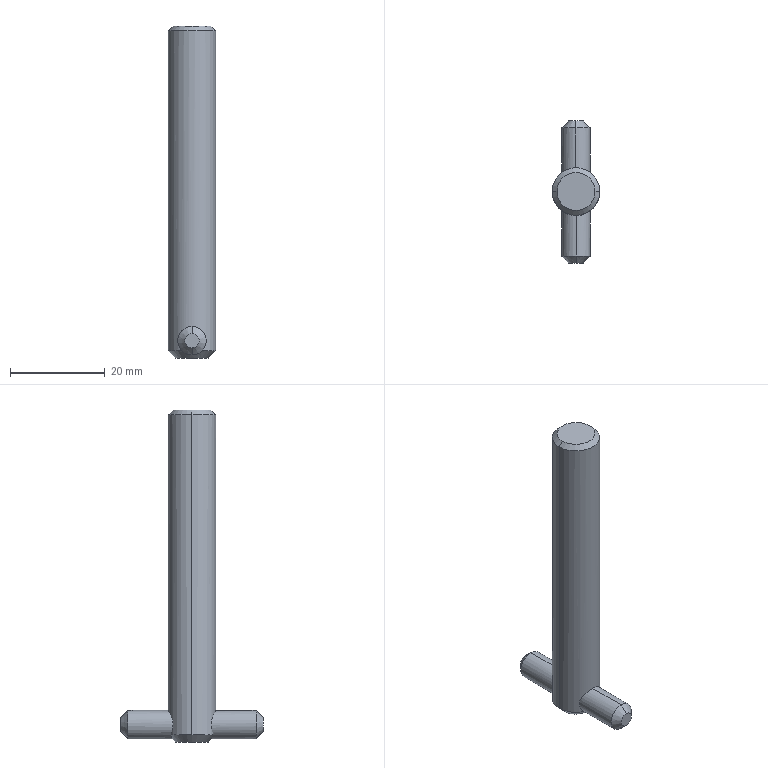Part | SolidWorks | features Chamfer 2, Extrusion 1, ICE 1 | 1 solid | 18 faces | box 10 x 30 x 70 mm | volume 5997 mm3 | cone 8 | cylinder 6 | plane 4 | commonest cylinder face diameters 6 x4 10 x2
STEP:
#1=CARTESIAN_POINT('',(4.,0.,70.));
#2=VERTEX_POINT('',#1);
#3=CARTESIAN_POINT('',(-4.,0.,70.));
#4=VERTEX_POINT('',#3);
#5=CARTESIAN_POINT('',(0.,0.,70.));
#6=DIRECTION('',(0.,0.,1.));
#7=DIRECTION('',(1.,0.,0.));
#8=AXIS2_PLACEMENT_3D('',#5,#6,#7);
#9=CIRCLE('',#8,4.);
#10=EDGE_CURVE('',#2,#4,#9,.T.);
#11=ORIENTED_EDGE('',*,*,#10,.F.);
#12=CARTESIAN_POINT('',(5.,0.,69.));
#13=VERTEX_POINT('',#12);
#14=CARTESIAN_POINT('',(4.,0.,70.));
#15=DIRECTION('',(0.7071,0.,-0.7071));
#16=VECTOR('',#15,1000.);
#17=LINE('',#14,#16);
#18=EDGE_CURVE('',#2,#13,#17,.T.);
#19=ORIENTED_EDGE('',*,*,#18,.T.);
#20=CARTESIAN_POINT('',(-5.,0.,69.));
#21=VERTEX_POINT('',#20);
#22=CARTESIAN_POINT('',(0.,0.,69.));
#23=DIRECTION('',(0.,0.,-1.));
#24=DIRECTION('',(1.,0.,0.));
#25=AXIS2_PLACEMENT_3D('',#22,#23,#24);
#26=CIRCLE('',#25,5.);
#27=EDGE_CURVE('',#21,#13,#26,.T.);
#28=ORIENTED_EDGE('',*,*,#27,.F.);
#29=CARTESIAN_POINT('',(-4.,0.,70.));
#30=DIRECTION('',(-0.7071,0.,-0.7071));
#31=VECTOR('',#30,1000.);
#32=LINE('',#29,#31);
#33=EDGE_CURVE('',#4,#21,#32,.T.);
#34=ORIENTED_EDGE('',*,*,#33,.F.);
#35=EDGE_LOOP('',(#11,#19,#28,#34));
#36=FACE_OUTER_BOUND('',#35,.T.);
#37=CARTESIAN_POINT('',(0.,0.,70.));
#38=DIRECTION('',(0.,0.,-1.));
#39=DIRECTION('',(-1.,0.,0.));
#40=AXIS2_PLACEMENT_3D('',#37,#38,#39);
#41=CONICAL_SURFACE('',#40,4.,0.7854);
#42=ADVANCED_FACE('',(#36),#41,.T.);
#43=CARTESIAN_POINT('',(0.,15.,5.144));
#44=VERTEX_POINT('',#43);
#45=CARTESIAN_POINT('',(0.,15.,2.144));
#46=VERTEX_POINT('',#45);
#47=CARTESIAN_POINT('',(0.,15.,3.644));
#48=DIRECTION('',(0.,1.,0.));
#49=DIRECTION('',(0.,0.,1.));
#50=AXIS2_PLACEMENT_3D('',#47,#48,#49);
#51=CIRCLE('',#50,1.5);
#52=EDGE_CURVE('',#44,#46,#51,.T.);
#53=ORIENTED_EDGE('',*,*,#52,.F.);
#54=CARTESIAN_POINT('',(0.,13.5,6.644));
#55=VERTEX_POINT('',#54);
#56=CARTESIAN_POINT('',(0.,15.,5.144));
#57=DIRECTION('',(0.,-0.7071,0.7071));
#58=VECTOR('',#57,1000.);
#59=LINE('',#56,#58);
#60=EDGE_CURVE('',#44,#55,#59,.T.);
#61=ORIENTED_EDGE('',*,*,#60,.T.);
#62=CARTESIAN_POINT('',(0.,13.5,0.6438));
#63=VERTEX_POINT('',#62);
#64=CARTESIAN_POINT('',(0.,13.5,3.644));
#65=DIRECTION('',(0.,-1.,0.));
#66=DIRECTION('',(0.,0.,1.));
#67=AXIS2_PLACEMENT_3D('',#64,#65,#66);
#68=CIRCLE('',#67,3.);
#69=EDGE_CURVE('',#63,#55,#68,.T.);
#70=ORIENTED_EDGE('',*,*,#69,.F.);
#71=CARTESIAN_POINT('',(0.,15.,2.144));
#72=DIRECTION('',(0.,-0.7071,-0.7071));
#73=VECTOR('',#72,1000.);
#74=LINE('',#71,#73);
#75=EDGE_CURVE('',#46,#63,#74,.T.);
#76=ORIENTED_EDGE('',*,*,#75,.F.);
#77=EDGE_LOOP('',(#53,#61,#70,#76));
#78=FACE_OUTER_BOUND('',#77,.T.);
#79=CARTESIAN_POINT('',(0.,15.,3.644));
#80=DIRECTION('',(0.,-1.,0.));
#81=DIRECTION('',(0.,0.,-1.));
#82=AXIS2_PLACEMENT_3D('',#79,#80,#81);
#83=CONICAL_SURFACE('',#82,1.5,0.7854);
#84=ADVANCED_FACE('',(#78),#83,.T.);
#85=CARTESIAN_POINT('',(-3.5,0.,0.));
#86=VERTEX_POINT('',#85);
#87=CARTESIAN_POINT('',(3.5,0.,0.));
#88=VERTEX_POINT('',#87);
#89=CARTESIAN_POINT('',(0.,0.,0.));
#90=DIRECTION('',(0.,0.,-1.));
#91=DIRECTION('',(1.,0.,0.));
#92=AXIS2_PLACEMENT_3D('',#89,#90,#91);
#93=CIRCLE('',#92,3.5);
#94=EDGE_CURVE('',#86,#88,#93,.T.);
#95=ORIENTED_EDGE('',*,*,#94,.F.);
#96=CARTESIAN_POINT('',(-5.,0.,1.5));
#97=VERTEX_POINT('',#96);
#98=CARTESIAN_POINT('',(-5.,0.,1.5));
#99=DIRECTION('',(-0.7071,0.,0.7071));
#100=VECTOR('',#99,1000.);
#101=LINE('',#98,#100);
#102=EDGE_CURVE('',#86,#97,#101,.T.);
#103=ORIENTED_EDGE('',*,*,#102,.T.);
#104=CARTESIAN_POINT('',(-2.099,4.538,1.5));
#105=VERTEX_POINT('',#104);
#106=CARTESIAN_POINT('',(0.,0.,1.5));
#107=DIRECTION('',(0.,0.,1.));
#108=DIRECTION('',(1.,0.,0.));
#109=AXIS2_PLACEMENT_3D('',#106,#107,#108);
#110=CIRCLE('',#109,5.);
#111=EDGE_CURVE('',#105,#97,#110,.T.);
#112=ORIENTED_EDGE('',*,*,#111,.F.);
#113=CARTESIAN_POINT('',(0.,4.144,0.6438));
#114=VERTEX_POINT('',#113);
#115=CARTESIAN_POINT('',(0.,4.144,0.6438));
#116=CARTESIAN_POINT('',(-0.1973,4.144,0.6438));
#117=CARTESIAN_POINT('',(-0.3976,4.149,0.6637));
#118=CARTESIAN_POINT('',(-0.7841,4.173,0.7414));
#119=CARTESIAN_POINT('',(-0.9715,4.191,0.7987));
#120=CARTESIAN_POINT('',(-1.334,4.248,0.9496));
#121=CARTESIAN_POINT('',(-1.507,4.288,1.043));
#122=CARTESIAN_POINT('',(-1.822,4.392,1.253));
#123=CARTESIAN_POINT('',(-1.968,4.458,1.372));
#124=CARTESIAN_POINT('',(-2.099,4.538,1.5));
#125=B_SPLINE_CURVE_WITH_KNOTS('',3,(#115,#116,#117,#118,#119,#120,#121,#122,#123,#124),.UNSPECIFIED.,.F.,.F.,(4,2,2,2,4),(0.002363,0.002953,0.003544,0.004135,0.004726),.UNSPECIFIED.);
#126=EDGE_CURVE('',#114,#105,#125,.T.);
#127=ORIENTED_EDGE('',*,*,#126,.F.);
#128=CARTESIAN_POINT('',(2.099,4.538,1.5));
#129=VERTEX_POINT('',#128);
#130=CARTESIAN_POINT('',(2.099,4.538,1.5));
#131=CARTESIAN_POINT('',(1.968,4.458,1.372));
#132=CARTESIAN_POINT('',(1.824,4.392,1.254));
#133=CARTESIAN_POINT('',(1.508,4.288,1.043));
#134=CARTESIAN_POINT('',(1.333,4.248,0.9493));
#135=CARTESIAN_POINT('',(0.7923,4.162,0.7241));
#136=CARTESIAN_POINT('',(0.3947,4.144,0.6438));
#137=CARTESIAN_POINT('',(0.,4.144,0.6438));
#138=B_SPLINE_CURVE_WITH_KNOTS('',3,(#130,#131,#132,#133,#134,#135,#136,#137),.UNSPECIFIED.,.F.,.F.,(4,2,2,4),(0.,0.0005907,0.001181,0.002363),.UNSPECIFIED.);
#139=EDGE_CURVE('',#129,#114,#138,.T.);
#140=ORIENTED_EDGE('',*,*,#139,.F.);
#141=CARTESIAN_POINT('',(5.,0.,1.5));
#142=VERTEX_POINT('',#141);
#143=CARTESIAN_POINT('',(0.,0.,1.5));
#144=DIRECTION('',(0.,0.,1.));
#145=DIRECTION('',(1.,0.,0.));
#146=AXIS2_PLACEMENT_3D('',#143,#144,#145);
#147=CIRCLE('',#146,5.);
#148=EDGE_CURVE('',#142,#129,#147,.T.);
#149=ORIENTED_EDGE('',*,*,#148,.F.);
#150=CARTESIAN_POINT('',(5.,0.,1.5));
#151=DIRECTION('',(0.7071,0.,0.7071));
#152=VECTOR('',#151,1000.);
#153=LINE('',#150,#152);
#154=EDGE_CURVE('',#88,#142,#153,.T.);
#155=ORIENTED_EDGE('',*,*,#154,.F.);
#156=EDGE_LOOP('',(#95,#103,#112,#127,#140,#149,#155));
#157=FACE_OUTER_BOUND('',#156,.T.);
#158=CARTESIAN_POINT('',(0.,0.,1.5));
#159=DIRECTION('',(0.,0.,1.));
#160=DIRECTION('',(1.,0.,0.));
#161=AXIS2_PLACEMENT_3D('',#158,#159,#160);
#162=CONICAL_SURFACE('',#161,5.,0.7854);
#163=ADVANCED_FACE('',(#157),#162,.T.);
#164=CARTESIAN_POINT('',(0.,-15.,2.144));
#165=VERTEX_POINT('',#164);
#166=CARTESIAN_POINT('',(0.,-15.,5.144));
#167=VERTEX_POINT('',#166);
#168=CARTESIAN_POINT('',(0.,-15.,3.644));
#169=DIRECTION('',(0.,-1.,0.));
#170=DIRECTION('',(0.,0.,1.));
#171=AXIS2_PLACEMENT_3D('',#168,#169,#170);
#172=CIRCLE('',#171,1.5);
#173=EDGE_CURVE('',#165,#167,#172,.T.);
#174=ORIENTED_EDGE('',*,*,#173,.F.);
#175=CARTESIAN_POINT('',(0.,-13.5,0.6438));
#176=VERTEX_POINT('',#175);
#177=CARTESIAN_POINT('',(0.,-13.5,0.6438));
#178=DIRECTION('',(0.,0.7071,-0.7071));
#179=VECTOR('',#178,1000.);
#180=LINE('',#177,#179);
#181=EDGE_CURVE('',#165,#176,#180,.T.);
#182=ORIENTED_EDGE('',*,*,#181,.T.);
#183=CARTESIAN_POINT('',(0.,-13.5,6.644));
#184=VERTEX_POINT('',#183);
#185=CARTESIAN_POINT('',(0.,-13.5,3.644));
#186=DIRECTION('',(0.,1.,0.));
#187=DIRECTION('',(0.,0.,1.));
#188=AXIS2_PLACEMENT_3D('',#185,#186,#187);
#189=CIRCLE('',#188,3.);
#190=EDGE_CURVE('',#184,#176,#189,.T.);
#191=ORIENTED_EDGE('',*,*,#190,.F.);
#192=CARTESIAN_POINT('',(0.,-13.5,6.644));
#193=DIRECTION('',(0.,0.7071,0.7071));
#194=VECTOR('',#193,1000.);
#195=LINE('',#192,#194);
#196=EDGE_CURVE('',#167,#184,#195,.T.);
#197=ORIENTED_EDGE('',*,*,#196,.F.);
#198=EDGE_LOOP('',(#174,#182,#191,#197));
#199=FACE_OUTER_BOUND('',#198,.T.);
#200=CARTESIAN_POINT('',(0.,-13.5,3.644));
#201=DIRECTION('',(0.,1.,0.));
#202=DIRECTION('',(0.,0.,1.));
#203=AXIS2_PLACEMENT_3D('',#200,#201,#202);
#204=CONICAL_SURFACE('',#203,3.,0.7854);
#205=ADVANCED_FACE('',(#199),#204,.T.);
#206=ORIENTED_EDGE('',*,*,#69,.T.);
#207=CARTESIAN_POINT('',(0.,5.,6.644));
#208=VERTEX_POINT('',#207);
#209=CARTESIAN_POINT('',(0.,15.,6.644));
#210=DIRECTION('',(0.,-1.,0.));
#211=VECTOR('',#210,1000.);
#212=LINE('',#209,#211);
#213=EDGE_CURVE('',#55,#208,#212,.T.);
#214=ORIENTED_EDGE('',*,*,#213,.T.);
#215=CARTESIAN_POINT('',(0.,5.,6.644));
#216=CARTESIAN_POINT('',(0.1527,5.,6.644));
#217=CARTESIAN_POINT('',(0.3036,4.993,6.632));
#218=CARTESIAN_POINT('',(0.6015,4.966,6.587));
#219=CARTESIAN_POINT('',(0.7498,4.946,6.553));
#220=CARTESIAN_POINT('',(1.037,4.893,6.463));
#221=CARTESIAN_POINT('',(1.175,4.862,6.408));
#222=CARTESIAN_POINT('',(1.44,4.79,6.28));
#223=CARTESIAN_POINT('',(1.569,4.749,6.205));
#224=CARTESIAN_POINT('',(1.931,4.619,5.958));
#225=CARTESIAN_POINT('',(2.144,4.522,5.763));
#226=CARTESIAN_POINT('',(2.51,4.33,5.313));
#227=CARTESIAN_POINT('',(2.658,4.237,5.066));
#228=CARTESIAN_POINT('',(2.828,4.124,4.657));
#229=CARTESIAN_POINT('',(2.875,4.091,4.514));
#230=CARTESIAN_POINT('',(2.947,4.039,4.225));
#231=CARTESIAN_POINT('',(2.973,4.02,4.076));
#232=CARTESIAN_POINT('',(3.001,3.999,3.772));
#233=CARTESIAN_POINT('',(3.004,3.997,3.619));
#234=CARTESIAN_POINT('',(2.986,4.01,3.317));
#235=CARTESIAN_POINT('',(2.966,4.026,3.168));
#236=CARTESIAN_POINT('',(2.871,4.094,2.723));
#237=CARTESIAN_POINT('',(2.766,4.169,2.445));
#238=CARTESIAN_POINT('',(2.481,4.344,1.932));
#239=CARTESIAN_POINT('',(2.306,4.442,1.703));
#240=CARTESIAN_POINT('',(2.099,4.538,1.5));
#241=B_SPLINE_CURVE_WITH_KNOTS('',3,(#215,#216,#217,#218,#219,#220,#221,#222,#223,#224,#225,#226,#227,#228,#229,#230,#231,#232,#233,#234,#235,#236,#237,#238,#239,#240),.UNSPECIFIED.,.F.,.F.,(4,2,2,2,2,2,2,2,2,2,2,2,4),(0.009625,0.01008,0.01053,0.01098,0.01144,0.01234,0.01325,0.0137,0.01415,0.0146,0.01506,0.01596,0.01687),.UNSPECIFIED.);
#242=EDGE_CURVE('',#208,#129,#241,.T.);
#243=ORIENTED_EDGE('',*,*,#242,.T.);
#244=ORIENTED_EDGE('',*,*,#139,.T.);
#245=CARTESIAN_POINT('',(0.,15.,0.6438));
#246=DIRECTION('',(0.,-1.,0.));
#247=VECTOR('',#246,1000.);
#248=LINE('',#245,#247);
#249=EDGE_CURVE('',#63,#114,#248,.T.);
#250=ORIENTED_EDGE('',*,*,#249,.F.);
#251=EDGE_LOOP('',(#206,#214,#243,#244,#250));
#252=FACE_OUTER_BOUND('',#251,.T.);
#253=CARTESIAN_POINT('',(0.,15.,3.644));
#254=DIRECTION('',(0.,-1.,0.));
#255=DIRECTION('',(0.,0.,-1.));
#256=AXIS2_PLACEMENT_3D('',#253,#254,#255);
#257=CYLINDRICAL_SURFACE('',#256,3.);
#258=ADVANCED_FACE('',(#252),#257,.T.);
#259=CARTESIAN_POINT('',(2.099,-4.538,1.5));
#260=VERTEX_POINT('',#259);
#261=CARTESIAN_POINT('',(0.,-5.,6.644));
#262=VERTEX_POINT('',#261);
#263=CARTESIAN_POINT('',(2.099,-4.538,1.5));
#264=CARTESIAN_POINT('',(2.304,-4.443,1.701));
#265=CARTESIAN_POINT('',(2.482,-4.343,1.935));
#266=CARTESIAN_POINT('',(2.693,-4.214,2.314));
#267=CARTESIAN_POINT('',(2.754,-4.173,2.446));
#268=CARTESIAN_POINT('',(2.859,-4.103,2.723));
#269=CARTESIAN_POINT('',(2.902,-4.072,2.868));
#270=CARTESIAN_POINT('',(2.965,-4.026,3.162));
#271=CARTESIAN_POINT('',(2.985,-4.011,3.311));
#272=CARTESIAN_POINT('',(3.004,-3.997,3.615));
#273=CARTESIAN_POINT('',(3.001,-3.999,3.77));
#274=CARTESIAN_POINT('',(2.959,-4.03,4.222));
#275=CARTESIAN_POINT('',(2.885,-4.086,4.518));
#276=CARTESIAN_POINT('',(2.66,-4.236,5.063));
#277=CARTESIAN_POINT('',(2.507,-4.331,5.316));
#278=CARTESIAN_POINT('',(2.143,-4.522,5.762));
#279=CARTESIAN_POINT('',(1.927,-4.621,5.961));
#280=CARTESIAN_POINT('',(1.567,-4.75,6.206));
#281=CARTESIAN_POINT('',(1.441,-4.79,6.279));
#282=CARTESIAN_POINT('',(1.176,-4.862,6.408));
#283=CARTESIAN_POINT('',(1.035,-4.894,6.464));
#284=CARTESIAN_POINT('',(0.7493,-4.946,6.553));
#285=CARTESIAN_POINT('',(0.6036,-4.966,6.586));
#286=CARTESIAN_POINT('',(0.3062,-4.993,6.632));
#287=CARTESIAN_POINT('',(0.1531,-5.,6.644));
#288=CARTESIAN_POINT('',(0.,-5.,6.644));
#289=B_SPLINE_CURVE_WITH_KNOTS('',3,(#263,#264,#265,#266,#267,#268,#269,#270,#271,#272,#273,#274,#275,#276,#277,#278,#279,#280,#281,#282,#283,#284,#285,#286,#287,#288),.UNSPECIFIED.,.F.,.F.,(4,2,2,2,2,2,2,2,2,2,2,2,4),(0.002367,0.003274,0.003728,0.004181,0.004635,0.005089,0.005996,0.006903,0.00781,0.008264,0.008718,0.009171,0.009625),.UNSPECIFIED.);
#290=EDGE_CURVE('',#260,#262,#289,.T.);
#291=ORIENTED_EDGE('',*,*,#290,.T.);
#292=CARTESIAN_POINT('',(0.,15.,6.644));
#293=DIRECTION('',(0.,-1.,0.));
#294=VECTOR('',#293,1000.);
#295=LINE('',#292,#294);
#296=EDGE_CURVE('',#262,#184,#295,.T.);
#297=ORIENTED_EDGE('',*,*,#296,.T.);
#298=ORIENTED_EDGE('',*,*,#190,.T.);
#299=CARTESIAN_POINT('',(0.,-4.144,0.6438));
#300=VERTEX_POINT('',#299);
#301=CARTESIAN_POINT('',(0.,15.,0.6438));
#302=DIRECTION('',(0.,-1.,0.));
#303=VECTOR('',#302,1000.);
#304=LINE('',#301,#303);
#305=EDGE_CURVE('',#300,#176,#304,.T.);
#306=ORIENTED_EDGE('',*,*,#305,.F.);
#307=CARTESIAN_POINT('',(0.,-4.144,0.6438));
#308=CARTESIAN_POINT('',(0.1973,-4.144,0.6438));
#309=CARTESIAN_POINT('',(0.3976,-4.149,0.6637));
#310=CARTESIAN_POINT('',(0.7841,-4.173,0.7414));
#311=CARTESIAN_POINT('',(0.9715,-4.191,0.7987));
#312=CARTESIAN_POINT('',(1.334,-4.248,0.9496));
#313=CARTESIAN_POINT('',(1.507,-4.288,1.043));
#314=CARTESIAN_POINT('',(1.822,-4.392,1.253));
#315=CARTESIAN_POINT('',(1.968,-4.458,1.372));
#316=CARTESIAN_POINT('',(2.099,-4.538,1.5));
#317=B_SPLINE_CURVE_WITH_KNOTS('',3,(#307,#308,#309,#310,#311,#312,#313,#314,#315,#316),.UNSPECIFIED.,.F.,.F.,(4,2,2,2,4),(0.002363,0.002953,0.003544,0.004135,0.004726),.UNSPECIFIED.);
#318=EDGE_CURVE('',#300,#260,#317,.T.);
#319=ORIENTED_EDGE('',*,*,#318,.T.);
#320=EDGE_LOOP('',(#291,#297,#298,#306,#319));
#321=FACE_OUTER_BOUND('',#320,.T.);
#322=CARTESIAN_POINT('',(0.,15.,3.644));
#323=DIRECTION('',(0.,-1.,0.));
#324=DIRECTION('',(0.,0.,-1.));
#325=AXIS2_PLACEMENT_3D('',#322,#323,#324);
#326=CYLINDRICAL_SURFACE('',#325,3.);
#327=ADVANCED_FACE('',(#321),#326,.T.);
#328=ORIENTED_EDGE('',*,*,#27,.T.);
#329=CARTESIAN_POINT('',(5.,0.,70.));
#330=DIRECTION('',(0.,0.,-1.));
#331=VECTOR('',#330,1000.);
#332=LINE('',#329,#331);
#333=EDGE_CURVE('',#13,#142,#332,.T.);
#334=ORIENTED_EDGE('',*,*,#333,.T.);
#335=ORIENTED_EDGE('',*,*,#148,.T.);
#336=ORIENTED_EDGE('',*,*,#242,.F.);
#337=CARTESIAN_POINT('',(-2.099,4.538,1.5));
#338=CARTESIAN_POINT('',(-2.304,4.443,1.701));
#339=CARTESIAN_POINT('',(-2.482,4.343,1.935));
#340=CARTESIAN_POINT('',(-2.693,4.214,2.314));
#341=CARTESIAN_POINT('',(-2.754,4.173,2.446));
#342=CARTESIAN_POINT('',(-2.859,4.103,2.723));
#343=CARTESIAN_POINT('',(-2.902,4.072,2.868));
#344=CARTESIAN_POINT('',(-2.965,4.026,3.162));
#345=CARTESIAN_POINT('',(-2.985,4.011,3.311));
#346=CARTESIAN_POINT('',(-3.004,3.997,3.615));
#347=CARTESIAN_POINT('',(-3.001,3.999,3.77));
#348=CARTESIAN_POINT('',(-2.959,4.03,4.222));
#349=CARTESIAN_POINT('',(-2.885,4.086,4.518));
#350=CARTESIAN_POINT('',(-2.66,4.236,5.063));
#351=CARTESIAN_POINT('',(-2.507,4.331,5.316));
#352=CARTESIAN_POINT('',(-2.143,4.522,5.762));
#353=CARTESIAN_POINT('',(-1.927,4.621,5.961));
#354=CARTESIAN_POINT('',(-1.567,4.75,6.206));
#355=CARTESIAN_POINT('',(-1.441,4.79,6.279));
#356=CARTESIAN_POINT('',(-1.176,4.862,6.408));
#357=CARTESIAN_POINT('',(-1.035,4.894,6.464));
#358=CARTESIAN_POINT('',(-0.7493,4.946,6.553));
#359=CARTESIAN_POINT('',(-0.6036,4.966,6.586));
#360=CARTESIAN_POINT('',(-0.3062,4.993,6.632));
#361=CARTESIAN_POINT('',(-0.1531,5.,6.644));
#362=CARTESIAN_POINT('',(0.,5.,6.644));
#363=B_SPLINE_CURVE_WITH_KNOTS('',3,(#337,#338,#339,#340,#341,#342,#343,#344,#345,#346,#347,#348,#349,#350,#351,#352,#353,#354,#355,#356,#357,#358,#359,#360,#361,#362),.UNSPECIFIED.,.F.,.F.,(4,2,2,2,2,2,2,2,2,2,2,2,4),(0.002367,0.003274,0.003728,0.004181,0.004635,0.005089,0.005996,0.006903,0.00781,0.008264,0.008718,0.009171,0.009625),.UNSPECIFIED.);
#364=EDGE_CURVE('',#105,#208,#363,.T.);
#365=ORIENTED_EDGE('',*,*,#364,.F.);
#366=ORIENTED_EDGE('',*,*,#111,.T.);
#367=CARTESIAN_POINT('',(-5.,0.,70.));
#368=DIRECTION('',(0.,0.,-1.));
#369=VECTOR('',#368,1000.);
#370=LINE('',#367,#369);
#371=EDGE_CURVE('',#21,#97,#370,.T.);
#372=ORIENTED_EDGE('',*,*,#371,.F.);
#373=EDGE_LOOP('',(#328,#334,#335,#336,#365,#366,#372));
#374=FACE_OUTER_BOUND('',#373,.T.);
#375=CARTESIAN_POINT('',(0.,0.,70.));
#376=DIRECTION('',(0.,0.,-1.));
#377=DIRECTION('',(-1.,0.,0.));
#378=AXIS2_PLACEMENT_3D('',#375,#376,#377);
#379=CYLINDRICAL_SURFACE('',#378,5.);
#380=ADVANCED_FACE('',(#374),#379,.T.);
#381=ORIENTED_EDGE('',*,*,#333,.F.);
#382=CARTESIAN_POINT('',(0.,0.,69.));
#383=DIRECTION('',(0.,0.,-1.));
#384=DIRECTION('',(1.,0.,0.));
#385=AXIS2_PLACEMENT_3D('',#382,#383,#384);
#386=CIRCLE('',#385,5.);
#387=EDGE_CURVE('',#13,#21,#386,.T.);
#388=ORIENTED_EDGE('',*,*,#387,.T.);
#389=ORIENTED_EDGE('',*,*,#371,.T.);
#390=CARTESIAN_POINT('',(-2.099,-4.538,1.5));
#391=VERTEX_POINT('',#390);
#392=CARTESIAN_POINT('',(0.,0.,1.5));
#393=DIRECTION('',(0.,0.,1.));
#394=DIRECTION('',(1.,0.,0.));
#395=AXIS2_PLACEMENT_3D('',#392,#393,#394);
#396=CIRCLE('',#395,5.);
#397=EDGE_CURVE('',#97,#391,#396,.T.);
#398=ORIENTED_EDGE('',*,*,#397,.T.);
#399=CARTESIAN_POINT('',(0.,-5.,6.644));
#400=CARTESIAN_POINT('',(-0.1527,-5.,6.644));
#401=CARTESIAN_POINT('',(-0.3036,-4.993,6.632));
#402=CARTESIAN_POINT('',(-0.6015,-4.966,6.587));
#403=CARTESIAN_POINT('',(-0.7498,-4.946,6.553));
#404=CARTESIAN_POINT('',(-1.037,-4.893,6.463));
#405=CARTESIAN_POINT('',(-1.175,-4.862,6.408));
#406=CARTESIAN_POINT('',(-1.44,-4.79,6.28));
#407=CARTESIAN_POINT('',(-1.569,-4.749,6.205));
#408=CARTESIAN_POINT('',(-1.931,-4.619,5.958));
#409=CARTESIAN_POINT('',(-2.144,-4.522,5.763));
#410=CARTESIAN_POINT('',(-2.51,-4.33,5.313));
#411=CARTESIAN_POINT('',(-2.658,-4.237,5.066));
#412=CARTESIAN_POINT('',(-2.828,-4.124,4.657));
#413=CARTESIAN_POINT('',(-2.875,-4.091,4.514));
#414=CARTESIAN_POINT('',(-2.947,-4.039,4.225));
#415=CARTESIAN_POINT('',(-2.973,-4.02,4.076));
#416=CARTESIAN_POINT('',(-3.001,-3.999,3.772));
#417=CARTESIAN_POINT('',(-3.004,-3.997,3.619));
#418=CARTESIAN_POINT('',(-2.986,-4.01,3.317));
#419=CARTESIAN_POINT('',(-2.966,-4.026,3.168));
#420=CARTESIAN_POINT('',(-2.871,-4.094,2.723));
#421=CARTESIAN_POINT('',(-2.766,-4.169,2.445));
#422=CARTESIAN_POINT('',(-2.481,-4.344,1.932));
#423=CARTESIAN_POINT('',(-2.306,-4.442,1.703));
#424=CARTESIAN_POINT('',(-2.099,-4.538,1.5));
#425=B_SPLINE_CURVE_WITH_KNOTS('',3,(#399,#400,#401,#402,#403,#404,#405,#406,#407,#408,#409,#410,#411,#412,#413,#414,#415,#416,#417,#418,#419,#420,#421,#422,#423,#424),.UNSPECIFIED.,.F.,.F.,(4,2,2,2,2,2,2,2,2,2,2,2,4),(0.009625,0.01008,0.01053,0.01098,0.01144,0.01234,0.01325,0.0137,0.01415,0.0146,0.01506,0.01596,0.01687),.UNSPECIFIED.);
#426=EDGE_CURVE('',#262,#391,#425,.T.);
#427=ORIENTED_EDGE('',*,*,#426,.F.);
#428=ORIENTED_EDGE('',*,*,#290,.F.);
#429=CARTESIAN_POINT('',(0.,0.,1.5));
#430=DIRECTION('',(0.,0.,1.));
#431=DIRECTION('',(1.,0.,0.));
#432=AXIS2_PLACEMENT_3D('',#429,#430,#431);
#433=CIRCLE('',#432,5.);
#434=EDGE_CURVE('',#260,#142,#433,.T.);
#435=ORIENTED_EDGE('',*,*,#434,.T.);
#436=EDGE_LOOP('',(#381,#388,#389,#398,#427,#428,#435));
#437=FACE_OUTER_BOUND('',#436,.T.);
#438=CARTESIAN_POINT('',(0.,0.,70.));
#439=DIRECTION('',(0.,0.,-1.));
#440=DIRECTION('',(-1.,0.,0.));
#441=AXIS2_PLACEMENT_3D('',#438,#439,#440);
#442=CYLINDRICAL_SURFACE('',#441,5.);
#443=ADVANCED_FACE('',(#437),#442,.T.);
#444=CARTESIAN_POINT('',(0.,0.,70.));
#445=DIRECTION('',(0.,0.,1.));
#446=DIRECTION('',(1.,0.,0.));
#447=AXIS2_PLACEMENT_3D('',#444,#445,#446);
#448=CIRCLE('',#447,4.);
#449=EDGE_CURVE('',#4,#2,#448,.T.);
#450=ORIENTED_EDGE('',*,*,#449,.T.);
#451=ORIENTED_EDGE('',*,*,#10,.T.);
#452=EDGE_LOOP('',(#450,#451));
#453=FACE_OUTER_BOUND('',#452,.T.);
#454=CARTESIAN_POINT('',(0.,0.,70.));
#455=DIRECTION('',(0.,0.,1.));
#456=DIRECTION('',(1.,0.,0.));
#457=AXIS2_PLACEMENT_3D('',#454,#455,#456);
#458=PLANE('',#457);
#459=ADVANCED_FACE('',(#453),#458,.T.);
#460=CARTESIAN_POINT('',(0.,0.,0.));
#461=DIRECTION('',(0.,0.,-1.));
#462=DIRECTION('',(1.,0.,0.));
#463=AXIS2_PLACEMENT_3D('',#460,#461,#462);
#464=CIRCLE('',#463,3.5);
#465=EDGE_CURVE('',#88,#86,#464,.T.);
#466=ORIENTED_EDGE('',*,*,#465,.T.);
#467=ORIENTED_EDGE('',*,*,#94,.T.);
#468=EDGE_LOOP('',(#466,#467));
#469=FACE_OUTER_BOUND('',#468,.T.);
#470=CARTESIAN_POINT('',(0.,0.,0.));
#471=DIRECTION('',(0.,0.,1.));
#472=DIRECTION('',(1.,0.,0.));
#473=AXIS2_PLACEMENT_3D('',#470,#471,#472);
#474=PLANE('',#473);
#475=ADVANCED_FACE('',(#469),#474,.F.);
#476=CARTESIAN_POINT('',(0.,-15.,3.644));
#477=DIRECTION('',(0.,-1.,0.));
#478=DIRECTION('',(0.,0.,1.));
#479=AXIS2_PLACEMENT_3D('',#476,#477,#478);
#480=CIRCLE('',#479,1.5);
#481=EDGE_CURVE('',#167,#165,#480,.T.);
#482=ORIENTED_EDGE('',*,*,#481,.T.);
#483=ORIENTED_EDGE('',*,*,#173,.T.);
#484=EDGE_LOOP('',(#482,#483));
#485=FACE_OUTER_BOUND('',#484,.T.);
#486=CARTESIAN_POINT('',(0.,-15.,3.644));
#487=DIRECTION('',(0.,1.,0.));
#488=DIRECTION('',(0.,0.,1.));
#489=AXIS2_PLACEMENT_3D('',#486,#487,#488);
#490=PLANE('',#489);
#491=ADVANCED_FACE('',(#485),#490,.F.);
#492=ORIENTED_EDGE('',*,*,#296,.F.);
#493=ORIENTED_EDGE('',*,*,#426,.T.);
#494=CARTESIAN_POINT('',(-2.099,-4.538,1.5));
#495=CARTESIAN_POINT('',(-1.968,-4.458,1.372));
#496=CARTESIAN_POINT('',(-1.824,-4.392,1.254));
#497=CARTESIAN_POINT('',(-1.508,-4.288,1.043));
#498=CARTESIAN_POINT('',(-1.333,-4.248,0.9493));
#499=CARTESIAN_POINT('',(-0.7923,-4.162,0.7241));
#500=CARTESIAN_POINT('',(-0.3947,-4.144,0.6438));
#501=CARTESIAN_POINT('',(0.,-4.144,0.6438));
#502=B_SPLINE_CURVE_WITH_KNOTS('',3,(#494,#495,#496,#497,#498,#499,#500,#501),.UNSPECIFIED.,.F.,.F.,(4,2,2,4),(0.,0.0005907,0.001181,0.002363),.UNSPECIFIED.);
#503=EDGE_CURVE('',#391,#300,#502,.T.);
#504=ORIENTED_EDGE('',*,*,#503,.T.);
#505=ORIENTED_EDGE('',*,*,#305,.T.);
#506=CARTESIAN_POINT('',(0.,-13.5,3.644));
#507=DIRECTION('',(0.,1.,0.));
#508=DIRECTION('',(0.,0.,1.));
#509=AXIS2_PLACEMENT_3D('',#506,#507,#508);
#510=CIRCLE('',#509,3.);
#511=EDGE_CURVE('',#176,#184,#510,.T.);
#512=ORIENTED_EDGE('',*,*,#511,.T.);
#513=EDGE_LOOP('',(#492,#493,#504,#505,#512));
#514=FACE_OUTER_BOUND('',#513,.T.);
#515=CARTESIAN_POINT('',(0.,15.,3.644));
#516=DIRECTION('',(0.,-1.,0.));
#517=DIRECTION('',(0.,0.,-1.));
#518=AXIS2_PLACEMENT_3D('',#515,#516,#517);
#519=CYLINDRICAL_SURFACE('',#518,3.);
#520=ADVANCED_FACE('',(#514),#519,.T.);
#521=ORIENTED_EDGE('',*,*,#213,.F.);
#522=CARTESIAN_POINT('',(0.,13.5,3.644));
#523=DIRECTION('',(0.,-1.,0.));
#524=DIRECTION('',(0.,0.,1.));
#525=AXIS2_PLACEMENT_3D('',#522,#523,#524);
#526=CIRCLE('',#525,3.);
#527=EDGE_CURVE('',#55,#63,#526,.T.);
#528=ORIENTED_EDGE('',*,*,#527,.T.);
#529=ORIENTED_EDGE('',*,*,#249,.T.);
#530=ORIENTED_EDGE('',*,*,#126,.T.);
#531=ORIENTED_EDGE('',*,*,#364,.T.);
#532=EDGE_LOOP('',(#521,#528,#529,#530,#531));
#533=FACE_OUTER_BOUND('',#532,.T.);
#534=CARTESIAN_POINT('',(0.,15.,3.644));
#535=DIRECTION('',(0.,-1.,0.));
#536=DIRECTION('',(0.,0.,-1.));
#537=AXIS2_PLACEMENT_3D('',#534,#535,#536);
#538=CYLINDRICAL_SURFACE('',#537,3.);
#539=ADVANCED_FACE('',(#533),#538,.T.);
#540=CARTESIAN_POINT('',(0.,15.,3.644));
#541=DIRECTION('',(0.,1.,0.));
#542=DIRECTION('',(0.,0.,1.));
#543=AXIS2_PLACEMENT_3D('',#540,#541,#542);
#544=CIRCLE('',#543,1.5);
#545=EDGE_CURVE('',#46,#44,#544,.T.);
#546=ORIENTED_EDGE('',*,*,#545,.T.);
#547=ORIENTED_EDGE('',*,*,#52,.T.);
#548=EDGE_LOOP('',(#546,#547));
#549=FACE_OUTER_BOUND('',#548,.T.);
#550=CARTESIAN_POINT('',(0.,15.,3.644));
#551=DIRECTION('',(0.,1.,0.));
#552=DIRECTION('',(0.,0.,1.));
#553=AXIS2_PLACEMENT_3D('',#550,#551,#552);
#554=PLANE('',#553);
#555=ADVANCED_FACE('',(#549),#554,.T.);
#556=ORIENTED_EDGE('',*,*,#181,.F.);
#557=ORIENTED_EDGE('',*,*,#481,.F.);
#558=ORIENTED_EDGE('',*,*,#196,.T.);
#559=ORIENTED_EDGE('',*,*,#511,.F.);
#560=EDGE_LOOP('',(#556,#557,#558,#559));
#561=FACE_OUTER_BOUND('',#560,.T.);
#562=CARTESIAN_POINT('',(0.,-13.5,3.644));
#563=DIRECTION('',(0.,1.,0.));
#564=DIRECTION('',(0.,0.,1.));
#565=AXIS2_PLACEMENT_3D('',#562,#563,#564);
#566=CONICAL_SURFACE('',#565,3.,0.7854);
#567=ADVANCED_FACE('',(#561),#566,.T.);
#568=ORIENTED_EDGE('',*,*,#102,.F.);
#569=ORIENTED_EDGE('',*,*,#465,.F.);
#570=ORIENTED_EDGE('',*,*,#154,.T.);
#571=ORIENTED_EDGE('',*,*,#434,.F.);
#572=ORIENTED_EDGE('',*,*,#318,.F.);
#573=ORIENTED_EDGE('',*,*,#503,.F.);
#574=ORIENTED_EDGE('',*,*,#397,.F.);
#575=EDGE_LOOP('',(#568,#569,#570,#571,#572,#573,#574));
#576=FACE_OUTER_BOUND('',#575,.T.);
#577=CARTESIAN_POINT('',(0.,0.,1.5));
#578=DIRECTION('',(0.,0.,1.));
#579=DIRECTION('',(1.,0.,0.));
#580=AXIS2_PLACEMENT_3D('',#577,#578,#579);
#581=CONICAL_SURFACE('',#580,5.,0.7854);
#582=ADVANCED_FACE('',(#576),#581,.T.);
#583=ORIENTED_EDGE('',*,*,#60,.F.);
#584=ORIENTED_EDGE('',*,*,#545,.F.);
#585=ORIENTED_EDGE('',*,*,#75,.T.);
#586=ORIENTED_EDGE('',*,*,#527,.F.);
#587=EDGE_LOOP('',(#583,#584,#585,#586));
#588=FACE_OUTER_BOUND('',#587,.T.);
#589=CARTESIAN_POINT('',(0.,15.,3.644));
#590=DIRECTION('',(0.,-1.,0.));
#591=DIRECTION('',(0.,0.,-1.));
#592=AXIS2_PLACEMENT_3D('',#589,#590,#591);
#593=CONICAL_SURFACE('',#592,1.5,0.7854);
#594=ADVANCED_FACE('',(#588),#593,.T.);
#595=ORIENTED_EDGE('',*,*,#18,.F.);
#596=ORIENTED_EDGE('',*,*,#449,.F.);
#597=ORIENTED_EDGE('',*,*,#33,.T.);
#598=ORIENTED_EDGE('',*,*,#387,.F.);
#599=EDGE_LOOP('',(#595,#596,#597,#598));
#600=FACE_OUTER_BOUND('',#599,.T.);
#601=CARTESIAN_POINT('',(0.,0.,70.));
#602=DIRECTION('',(0.,0.,-1.));
#603=DIRECTION('',(-1.,0.,0.));
#604=AXIS2_PLACEMENT_3D('',#601,#602,#603);
#605=CONICAL_SURFACE('',#604,4.,0.7854);
#606=ADVANCED_FACE('',(#600),#605,.T.);
#607=CLOSED_SHELL('',(#42,#84,#163,#205,#258,#327,#380,#443,#459,#475,#491,#520,#539,#555,#567,#582,#594,#606));
#608=MANIFOLD_SOLID_BREP('',#607);
#609=CARTESIAN_POINT('',(0.,0.,0.));
#610=DIRECTION('',(0.,0.,1.));
#611=DIRECTION('',(1.,0.,0.));
#612=AXIS2_PLACEMENT_3D('',#609,#610,#611);
#613=(LENGTH_UNIT()NAMED_UNIT(*)SI_UNIT(.MILLI.,.METRE.));
#614=UNCERTAINTY_MEASURE_WITH_UNIT(LENGTH_MEASURE(0.00001),#613,'','');
#615=(NAMED_UNIT(*)PLANE_ANGLE_UNIT()SI_UNIT($,.RADIAN.));
#616=(NAMED_UNIT(*)SI_UNIT($,.STERADIAN.)SOLID_ANGLE_UNIT());
#617=(GEOMETRIC_REPRESENTATION_CONTEXT(3)GLOBAL_UNCERTAINTY_ASSIGNED_CONTEXT((#614))GLOBAL_UNIT_ASSIGNED_CONTEXT((#613,#615,#616))REPRESENTATION_CONTEXT('',''));
#618=ADVANCED_BREP_SHAPE_REPRESENTATION('',(#608,#612),#617);